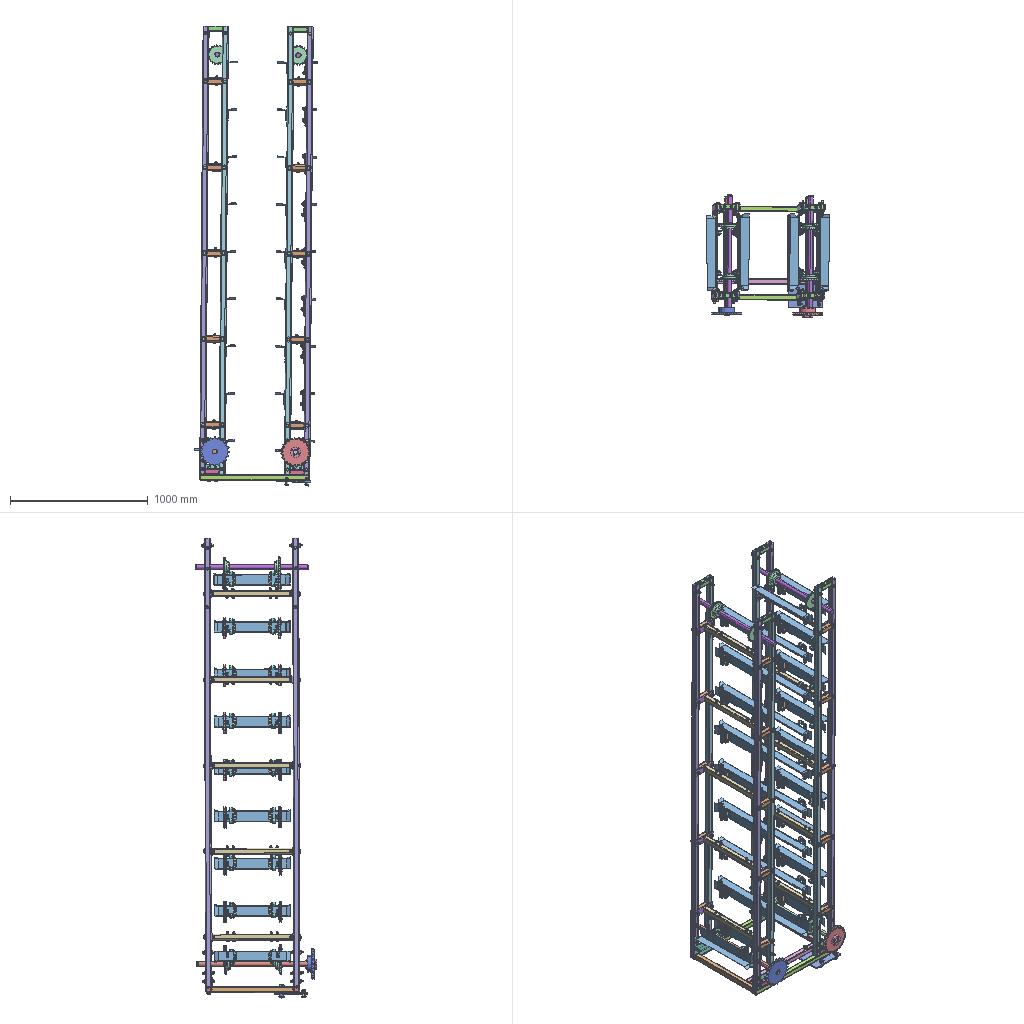Assembly | STEP file | 56 different items | 2795 placed | box 888 x 883 x 3334 mm
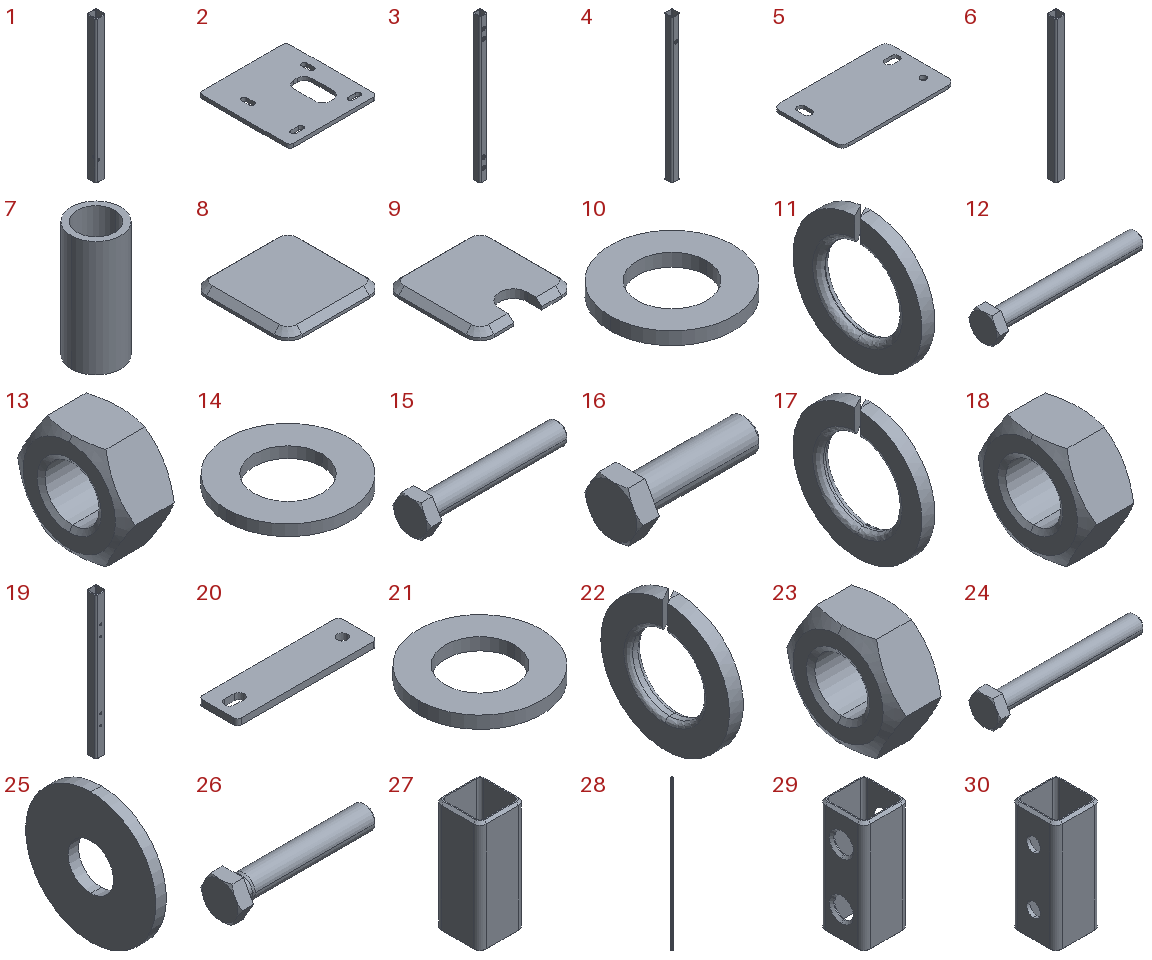Parts list (item | name | quantity | parent item | size | volume):
1 | IN-01-01-01-05 | x1 | in IN-01-01-01 | 40 x 40 x 590 mm | 239994 mm3
2 | IN-01-01-01-08 | x1 | in IN-01-01-01 | 240 x 250 x 10 mm | 535218 mm3
3 | IN-01-01-01-07 | x2 | in IN-01-01-01 | 40 x 40 x 795 mm | 317936 mm3
4 | IN-01-01-01-04 | x1 | in IN-01-01-01 | 40 x 40 x 715 mm | 290473 mm3
5 | IN-01-01-01-01 | x4 | in IN-01-01-01 | 180 x 110 x 5 mm | 95551 mm3
6 | IN-01-01-01-06 | x1 | in IN-01-01-01 | 40 x 40 x 590 mm | 240323 mm3
7 | IN-01-01-01-09 | x28 | in IN-01-01-01, IN-01-01-04 | 17.2 x 17.2 x 40 mm | 3820 mm3
8 | IN-01-01-01-03 | x10 | in IN-01-01-01, IN-01-01-04 | 34 x 34 x 3 mm | 3157 mm3
9 | IN-01-01-01-02 | x2 | in IN-01-01-01 | 34 x 34 x 3 mm | 2909 mm3
10 | DIN 126 - 13,5 | x120 | in IN-01-01-01, IN-01-01-03, IN-01-01-04 | 24 x 24 x 2.5 mm | 773.126 mm3
11 | DIN 128 - A12 | x80 | in IN-01-01-01, IN-01-01-03, IN-01-01-04 | 2.1 x 21.1 x 21.1 mm | 443.515 mm3
12 | DIN 931-1 - M12 x 100 | x8 | in IN-01-01-01 | 107.5 x 21.939 x 19 mm | 13582 mm3
13 | DIN 934 - M12 x 1,75 | x80 | in IN-01-01-01, IN-01-01-03, IN-01-01-04 | 10 x 21.939 x 19 mm | 2235 mm3
14 | DIN 126 - 15,5 | x8 | in IN-01-01-01 | 28 x 28 x 2.5 mm | 1068 mm3
15 | DIN 931-1 - M14 x 90 | x2 | in IN-01-01-01 | 98.8 x 25.403 x 22 mm | 17447 mm3
16 | DIN 931-1 - M14 x 50 | x2 | in IN-01-01-01 | 58.8 x 25.403 x 22 mm | 11289 mm3
17 | DIN 128 - A14 | x4 | in IN-01-01-01 | 2.4 x 24.1 x 24.1 mm | 656.657 mm3
18 | DIN 934 - M14 x 2 | x4 | in IN-01-01-01 | 11 x 25.403 x 22 mm | 3279 mm3
19 | IN-01-01-03-01 | x10 | in IN-01-01-03 | 40 x 40 x 584 mm | 236623 mm3
20 | IN-01-01-03-02 | x20 | in IN-01-01-03 | 180 x 50 x 8 mm | 68457 mm3
21 | DIN 126 - 9 | x80 | in IN-01-01-03 | 16 x 16 x 1.6 mm | 219.911 mm3
22 | DIN 128 - A8 | x40 | in IN-01-01-03 | 1.6 x 14.8 x 14.8 mm | 178.354 mm3
23 | DIN 934 - M8 x 1,25 | x40 | in IN-01-01-03 | 6.5 x 15.011 x 13 mm | 685.44 mm3
24 | DIN 931-1 - M8 x 65 | x40 | in IN-01-01-03 | 70.3 x 15.011 x 13 mm | 4009 mm3
25 | DIN 9021 - 13 | x40 | in IN-01-01-03 | 3 x 37 x 37 mm | 2827 mm3
26 | DIN 933 - M12  x 70 | x40 | in IN-01-01-03 | 77.5 x 21.939 x 19 mm | 10105 mm3
27 | IN-01-01-04-03 | x20 | in IN-01-01-04 | 40 x 40 x 100 mm | 40287 mm3
28 | IN-01-01-04-02 | x4 | in IN-01-01-04 | 40 x 40 x 3250 mm | 1317285 mm3
29 | IN-01-01-04-05 | x4 | in IN-01-01-04 | 40 x 40 x 100 mm | 37023 mm3
30 | IN-01-01-04-04 | x4 | in IN-01-01-04 | 40 x 40 x 100 mm | 38931 mm3
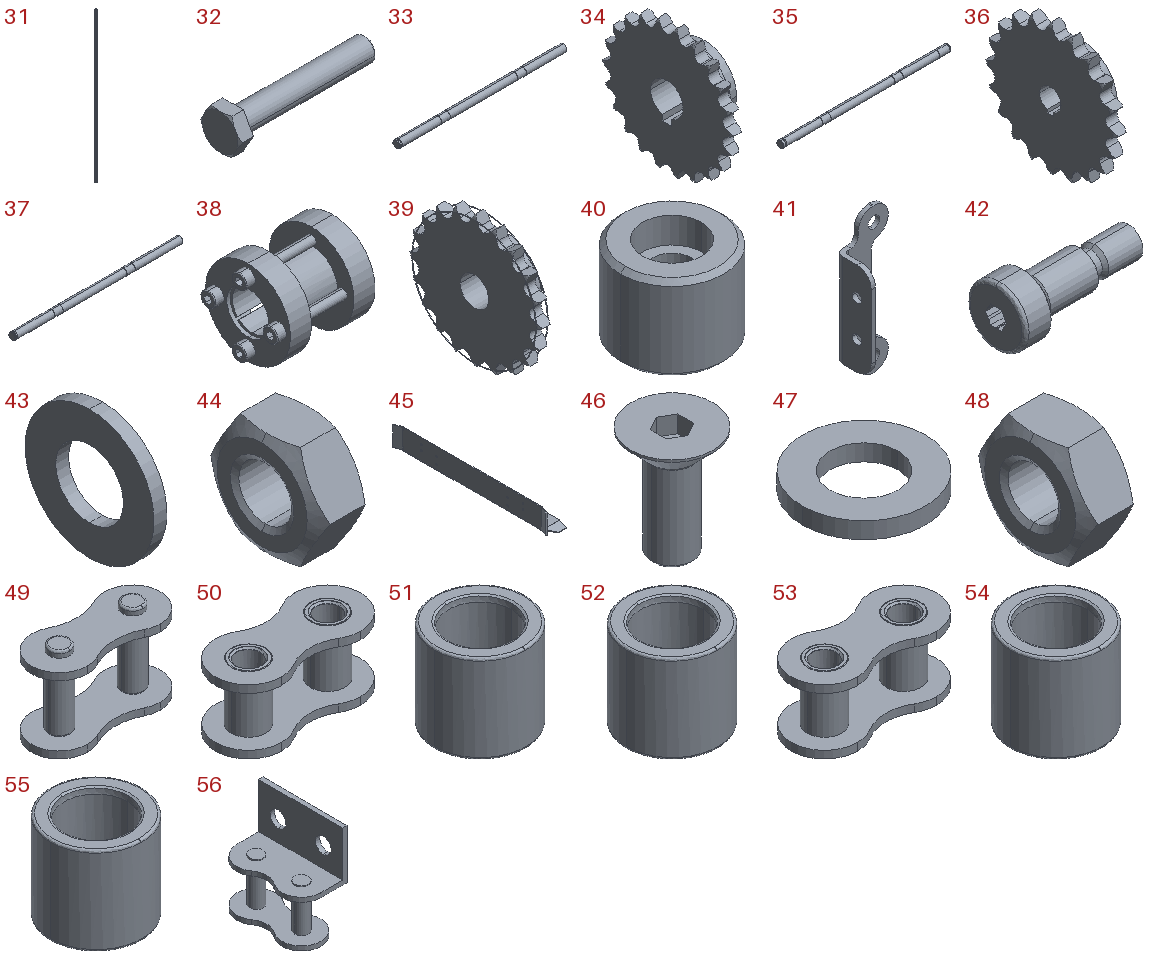31 | IN-01-01-04-01 | x4 | in IN-01-01-04 | 40 x 40 x 3250 mm | 1322181 mm3
32 | DIN 931-1 - M12 x 70 | x32 | in IN-01-01-04 | 77.5 x 21.939 x 19 mm | 10189 mm3
33 | IN-01-09-01 | x2 | in IN-01-09 | 816.1 x 35 x 35 mm | 780993 mm3
34 | IN-01-09-02 | x8 | in IN-01-09, IN-01-20, IN-01-21 | 40 x 141.8 x 140.357 mm | 249105 mm3
35 | IN-01-20-01_1 | x1 | in IN-01-20-01 | 865 x 35 x 35 mm | 826460 mm3
36 | IN-01-20-02 | x1 | in IN-01-20 | 50 x 218.1 x 218.1 mm | 860635 mm3
37 | IN-01-21-01 | x1 | in IN-01-21 | 865 x 35 x 35 mm | 828041 mm3
38 | IN-01-21-03 | x1 | in IN-01-21-02 | 83 x 75 x 75 mm | 165688 mm3
39 | IN-01-21-02_1 | x1 | in IN-01-21-02 | - | -
40 | IN-01-08-01-02-02 | x112 | in IN-01-08-01-02 | 28 x 28 x 23 mm | 11236 mm3
41 | IN-01-08-01-02-01 | x56 | in IN-01-08-01-02 | 34 x 25 x 101 mm | 9812 mm3
42 | ANSI B18.3.3M - M8x1,25 x 29,25 | x112 | in IN-01-08-01-02 | 36.25 x 16 x 16 mm | 3128 mm3
43 | DIN 125-2 - B 8,4 | x112 | in IN-01-08-01-02 | 1.6 x 16 x 16 mm | 233.031 mm3
44 | DIN 934 - M8 | x112 | in IN-01-08-01-02 | 6.5 x 15.011 x 13 mm | 685.44 mm3
45 | IN-01-08-01-01_1 | x28 | in IN-01-08-01-01 | 74.017 x 548.705 x 83.447 mm | 217025 mm3
46 | DIN 7991 - M6x16 | x224 | in IN-01-08-01-01, IN-01-08-01 | 12 x 12 x 16 mm | 554.104 mm3
47 | DIN 126 - 6,6 | x224 | in IN-01-08-01-01, IN-01-08-01 | 12 x 12 x 1.6 mm | 126.217 mm3
48 | DIN 934 - M6 x 1 | x224 | in IN-01-08-01-01, IN-01-08-01 | 5 x 11.547 x 10 mm | 321.226 mm3
49 | 12b-1_01 | x112 | in IN_01_01_07_01_02 | 33.5 x 14.5 x 22.6 mm | 2362 mm3
50 | 12b-1_02 | x112 | in IN_01_01_07_01_02 | 35 x 15.9 x 15.6 mm | 2056 mm3
51 | 12b-1_03 | x112 | in IN_01_01_07_01_02 | 12.07 x 12.07 x 11.6 mm | 689.728 mm3
52 | 12b-1_04 | x112 | in IN_01_01_07_01_02 | 12.07 x 12.07 x 11.6 mm | 689.728 mm3
53 | 12b-1_05 | x112 | in IN_01_01_07_01_02 | 35 x 15.9 x 15.6 mm | 2056 mm3
54 | 12b-1_06 | x112 | in IN_01_01_07_01_02 | 12.07 x 12.07 x 11.6 mm | 689.728 mm3
55 | 12b-1_07 | x112 | in IN_01_01_07_01_02 | 12.07 x 12.07 x 11.6 mm | 689.728 mm3
56 | IN_01_01_07_01_03 | x56 | in IN-01-08-01-02_1 | 19.15 x 35.35 x 39.1 mm | 3982 mm3
Placements (level | parent | child | x y z in mm | rotation matrix by rows), first 376 of 3099 lines:
1 | subassembly 2 | R1 | 7951.862 -633.159 955.539 | 1 0 0 0 1 0 0 0 1
2 | R1 | IN-01-01-01 | -8275.879 162.941 -2741.192 | -0.005068 -0.007537 1 -1 -0.002503 -0.005087 0.002541 -1 -0.007524
3 | IN-01-01-01 | IN-01-01-01-05 | -169.23 -114.088 623.28 | 0 0 -1 0 1 0 1 0 0
3 | IN-01-01-01 | IN-01-01-01-08 | -369.23 -94.088 343.28 | 1 0 0 0 0 1 0 -1 -0
3 | IN-01-01-01 | IN-01-01-01-07 | -784.23 -114.088 -111.72 | 1 0 0 0 1 0 0 0 1
3 | IN-01-01-01 | IN-01-01-01-07 | -144.23 -114.088 683.28 | -1 0 0 0 1 0 0 0 -1
3 | IN-01-01-01 | IN-01-01-01-04 | -259.23 -114.088 -71.72 | 1 0 0 0 1 0 0 0 1
3 | IN-01-01-01 | IN-01-01-01-01 | -164.23 -204.088 68.28 | 0 0 -1 0 -1 0 -1 0 0
3 | IN-01-01-01 | IN-01-01-01-01 | -169.23 -204.088 503.28 | 0 0 1 0 -1 0 1 0 -0
3 | IN-01-01-01 | IN-01-01-01-01 | -764.23 -204.088 503.28 | 0 0 1 0 -1 0 1 0 -0
3 | IN-01-01-01 | IN-01-01-01-01 | -759.23 -204.088 68.28 | 0 0 -1 0 -1 0 -1 0 0
3 | IN-01-01-01 | IN-01-01-01-06 | -169.23 -114.088 -91.72 | 0 0 -1 0 1 0 1 0 0
3 | IN-01-01-01 | IN-01-01-01-09 | -784.23 -134.088 -46.72 | 1 0 0 0 0 1 0 -1 0
3 | IN-01-01-01 | IN-01-01-01-09 | -784.23 -134.088 3.28 | 1 0 0 0 0 1 0 -1 0
3 | IN-01-01-01 | IN-01-01-01-09 | -784.23 -134.088 618.28 | 1 0 0 0 0 1 0 -1 0
3 | IN-01-01-01 | IN-01-01-01-09 | -144.23 -134.088 3.28 | 1 0 0 0 0 1 0 -1 0
3 | IN-01-01-01 | IN-01-01-01-09 | -144.23 -134.088 618.28 | 1 0 0 0 0 1 0 -1 0
3 | IN-01-01-01 | IN-01-01-01-09 | -144.23 -134.088 568.28 | 1 0 0 0 0 1 0 -1 0
3 | IN-01-01-01 | IN-01-01-01-09 | -144.23 -134.088 -46.72 | 1 0 0 0 0 1 0 -1 0
3 | IN-01-01-01 | IN-01-01-01-09 | -784.23 -134.088 568.28 | 1 0 0 0 0 1 0 -1 0
3 | IN-01-01-01 | IN-01-01-01-03 | -161.33 -131.188 680.28 | 0 -1 0 1 0 0 0 0 1
3 | IN-01-01-01 | IN-01-01-01-02 | -127.13 -97.188 -108.72 | -1 0 0 0 1 0 0 0 -1
3 | IN-01-01-01 | IN-01-01-01-03 | -801.33 -131.188 680.28 | 0 -1 0 1 0 0 0 0 1
3 | IN-01-01-01 | IN-01-01-01-02 | -767.33 -97.188 -108.72 | -1 0 0 0 1 0 0 0 -1
3 | IN-01-01-01 | DIN 126 - 13,5 | -784.23 -91.588 568.28 | -1 0 0 0 0 1 0 1 0
3 | IN-01-01-01 | DIN 126 - 13,5 | -784.23 -91.588 -46.72 | -1 0 0 0 0 1 0 1 0
3 | IN-01-01-01 | DIN 126 - 13,5 | -784.23 -91.588 3.28 | -1 0 0 0 0 1 0 1 0
3 | IN-01-01-01 | DIN 126 - 13,5 | -784.23 -91.588 618.28 | -1 0 0 0 0 1 0 1 0
3 | IN-01-01-01 | DIN 126 - 13,5 | -144.23 -91.588 3.28 | -1 0 0 0 0 1 0 1 0
3 | IN-01-01-01 | DIN 126 - 13,5 | -144.23 -91.588 618.28 | -1 0 0 0 0 1 0 1 0
3 | IN-01-01-01 | DIN 126 - 13,5 | -144.23 -91.588 568.28 | -1 0 0 0 0 1 0 1 0
3 | IN-01-01-01 | DIN 126 - 13,5 | -144.23 -91.588 -46.72 | -1 0 0 0 0 1 0 1 0
3 | IN-01-01-01 | DIN 126 - 13,5 | -144.23 -176.588 618.28 | 1 0 0 0 0 -1 0 1 -0
3 | IN-01-01-01 | DIN 126 - 13,5 | -144.23 -176.588 -46.72 | 1 0 0 0 0 -1 0 1 -0
3 | IN-01-01-01 | DIN 126 - 13,5 | -144.23 -176.588 3.28 | 1 0 0 0 0 -1 0 1 -0
3 | IN-01-01-01 | DIN 126 - 13,5 | -144.23 -176.588 568.28 | 1 0 0 0 0 -1 0 1 -0
3 | IN-01-01-01 | DIN 126 - 13,5 | -784.23 -176.588 618.28 | 1 0 0 0 0 -1 0 1 -0
3 | IN-01-01-01 | DIN 126 - 13,5 | -784.23 -176.588 568.28 | 1 0 0 0 0 -1 0 1 -0
3 | IN-01-01-01 | DIN 126 - 13,5 | -784.23 -176.588 3.28 | 1 0 0 0 0 -1 0 1 -0
3 | IN-01-01-01 | DIN 126 - 13,5 | -784.23 -176.588 -46.72 | 1 0 0 0 0 -1 0 1 -0
3 | IN-01-01-01 | DIN 128 - A12 | -144.23 -176.588 618.28 | 0 1 0 -1 0 0 0 0 1
3 | IN-01-01-01 | DIN 128 - A12 | -144.23 -176.588 568.28 | 0 1 0 -1 0 0 0 0 1
3 | IN-01-01-01 | DIN 128 - A12 | -144.23 -176.588 3.28 | 0 1 0 -1 0 0 0 0 1
3 | IN-01-01-01 | DIN 128 - A12 | -144.23 -176.588 -46.72 | 0 1 0 -1 0 0 0 0 1
3 | IN-01-01-01 | DIN 128 - A12 | -784.23 -176.588 -46.72 | 0 1 0 -1 0 0 0 0 1
3 | IN-01-01-01 | DIN 128 - A12 | -784.23 -176.588 3.28 | 0 1 0 -1 0 0 0 0 1
3 | IN-01-01-01 | DIN 128 - A12 | -784.23 -176.588 568.28 | 0 1 0 -1 0 0 0 0 1
3 | IN-01-01-01 | DIN 128 - A12 | -784.23 -176.588 618.28 | 0 1 0 -1 0 0 0 0 1
3 | IN-01-01-01 | DIN 931-1 - M12 x 100 | -784.23 -91.588 -46.72 | 0 1 0 -1 0 0 0 0 1
3 | IN-01-01-01 | DIN 931-1 - M12 x 100 | -784.23 -91.588 3.28 | 0 1 0 -1 0 0 0 0 1
3 | IN-01-01-01 | DIN 931-1 - M12 x 100 | -784.23 -91.588 568.28 | 0 1 0 -1 0 0 0 0 1
3 | IN-01-01-01 | DIN 931-1 - M12 x 100 | -784.23 -91.588 618.28 | 0 1 0 -1 0 0 0 0 1
3 | IN-01-01-01 | DIN 931-1 - M12 x 100 | -144.23 -91.588 618.28 | 0 1 0 -1 0 0 0 0 1
3 | IN-01-01-01 | DIN 931-1 - M12 x 100 | -144.23 -91.588 568.28 | 0 1 0 -1 0 0 0 0 1
3 | IN-01-01-01 | DIN 931-1 - M12 x 100 | -144.23 -91.588 3.28 | 0 1 0 -1 0 0 0 0 1
3 | IN-01-01-01 | DIN 931-1 - M12 x 100 | -144.23 -91.588 -46.72 | 0 1 0 -1 0 0 0 0 1
3 | IN-01-01-01 | DIN 934 - M12 x 1,75 | -144.23 -188.688 618.28 | 0 -1 0 1 0 0 0 0 1
3 | IN-01-01-01 | DIN 934 - M12 x 1,75 | -144.23 -188.688 568.28 | 0 -1 0 1 0 0 0 0 1
3 | IN-01-01-01 | DIN 934 - M12 x 1,75 | -144.23 -188.688 3.28 | 0 -1 0 1 0 0 0 0 1
3 | IN-01-01-01 | DIN 934 - M12 x 1,75 | -144.23 -188.688 -46.72 | 0 -1 0 1 0 0 0 0 1
3 | IN-01-01-01 | DIN 934 - M12 x 1,75 | -784.23 -188.688 -46.72 | 0 -1 0 1 0 0 0 0 1
3 | IN-01-01-01 | DIN 934 - M12 x 1,75 | -784.23 -188.688 3.28 | 0 -1 0 1 0 0 0 0 1
3 | IN-01-01-01 | DIN 934 - M12 x 1,75 | -784.23 -188.688 568.28 | 0 -1 0 1 0 0 0 0 1
3 | IN-01-01-01 | DIN 934 - M12 x 1,75 | -784.23 -188.688 618.28 | 0 -1 0 1 0 0 0 0 1
3 | IN-01-01-01 | DIN 126 - 15,5 | -261.73 -64.588 520.78 | -1 0 0 0 0 1 0 1 -0
3 | IN-01-01-01 | DIN 126 - 15,5 | -251.73 -64.588 665.78 | -1 0 0 0 0 1 0 1 -0
3 | IN-01-01-01 | DIN 126 - 15,5 | -93.73 -64.588 665.78 | -1 0 0 0 0 1 0 1 -0
3 | IN-01-01-01 | DIN 126 - 15,5 | -96.73 -64.588 520.78 | -1 0 0 0 0 1 0 1 -0
3 | IN-01-01-01 | DIN 931-1 - M14 x 90 | -261.73 -64.588 520.78 | 0 1 0 -1 0 0 0 0 1
3 | IN-01-01-01 | DIN 931-1 - M14 x 90 | -251.73 -64.588 665.78 | 0 1 0 -1 0 0 0 0 1
3 | IN-01-01-01 | DIN 931-1 - M14 x 50 | -93.73 -64.588 665.78 | 0 1 0 -1 0 0 0 0 1
3 | IN-01-01-01 | DIN 931-1 - M14 x 50 | -96.73 -64.588 520.78 | 0 1 0 -1 0 0 0 0 1
3 | IN-01-01-01 | DIN 126 - 15,5 | -93.73 -96.588 665.78 | 1 0 0 0 0 -1 0 1 -0
3 | IN-01-01-01 | DIN 126 - 15,5 | -251.73 -136.588 665.78 | 1 0 0 0 0 -1 0 1 -0
3 | IN-01-01-01 | DIN 126 - 15,5 | -261.73 -136.588 520.78 | 1 0 0 0 0 -1 0 1 -0
3 | IN-01-01-01 | DIN 126 - 15,5 | -96.73 -96.588 520.78 | 1 0 0 0 0 -1 0 1 -0
3 | IN-01-01-01 | DIN 128 - A14 | -93.73 -96.588 665.78 | 0 1 0 -1 0 0 0 0 1
3 | IN-01-01-01 | DIN 128 - A14 | -251.73 -136.588 665.78 | 0 1 0 -1 0 0 0 0 1
3 | IN-01-01-01 | DIN 128 - A14 | -261.73 -136.588 520.78 | 0 1 0 -1 0 0 0 0 1
3 | IN-01-01-01 | DIN 128 - A14 | -96.73 -96.588 520.78 | 0 1 0 -1 0 0 0 0 1
3 | IN-01-01-01 | DIN 934 - M14 x 2 | -96.73 -109.988 520.78 | 0 -1 0 1 0 0 0 0 1
3 | IN-01-01-01 | DIN 934 - M14 x 2 | -93.73 -109.988 665.78 | 0 -1 0 1 0 0 0 0 1
3 | IN-01-01-01 | DIN 934 - M14 x 2 | -251.73 -149.988 665.78 | 0 -1 0 1 0 0 0 0 1
3 | IN-01-01-01 | DIN 934 - M14 x 2 | -261.73 -149.988 520.78 | 0 -1 0 1 0 0 0 0 1
2 | R1 | IN-01-01-03 | -8254.616 637.893 -1630.668 | 1 -0.007537 0.005068 -0.005087 -0.002503 1 -0.007524 -1 -0.002541
3 | IN-01-01-03 | IN-01-01-03-01 | -22.21 -4.25 -300.0 | 1 0 0 0 1 0 0 0 1
3 | IN-01-01-03 | IN-01-01-03-02 | -122.21 20.75 284.0 | 1 0 0 0 1 0 0 0 1
3 | IN-01-01-03 | IN-01-01-03-02 | -122.21 -29.25 -300.0 | 1 0 0 0 -1 0 0 0 -1
3 | IN-01-01-03 | DIN 126 - 9 | -22.21 21.35 172.0 | -1 0 0 0 0 1 0 1 0
3 | IN-01-01-03 | DIN 126 - 9 | -22.21 21.35 -144.0 | -1 0 0 0 0 1 0 1 0
3 | IN-01-01-03 | DIN 126 - 9 | -22.21 21.35 128.0 | -1 0 0 0 0 1 0 1 0
3 | IN-01-01-03 | DIN 126 - 9 | -22.21 21.35 -188.0 | -1 0 0 0 0 1 0 1 0
3 | IN-01-01-03 | DIN 126 - 9 | -22.21 -29.85 172.0 | 1 0 0 0 0 -1 0 1 0
3 | IN-01-01-03 | DIN 126 - 9 | -22.21 -29.85 -144.0 | 1 0 0 0 0 -1 0 1 0
3 | IN-01-01-03 | DIN 126 - 9 | -22.21 -29.85 128.0 | 1 0 0 0 0 -1 0 1 0
3 | IN-01-01-03 | DIN 126 - 9 | -22.21 -29.85 -188.0 | 1 0 0 0 0 -1 0 1 0
3 | IN-01-01-03 | DIN 128 - A8 | -22.21 -29.85 172.0 | 0 1 0 -1 0 0 0 0 1
3 | IN-01-01-03 | DIN 128 - A8 | -22.21 -29.85 -144.0 | 0 1 0 -1 0 0 0 0 1
3 | IN-01-01-03 | DIN 128 - A8 | -22.21 -29.85 128.0 | 0 1 0 -1 0 0 0 0 1
3 | IN-01-01-03 | DIN 128 - A8 | -22.21 -29.85 -188.0 | 0 1 0 -1 0 0 0 0 1
3 | IN-01-01-03 | DIN 934 - M8 x 1,25 | -22.21 -37.95 172.0 | 0 -1 0 1 0 0 0 0 1
3 | IN-01-01-03 | DIN 934 - M8 x 1,25 | -22.21 -37.95 128.0 | 0 -1 0 1 0 0 0 0 1
3 | IN-01-01-03 | DIN 934 - M8 x 1,25 | -22.21 -37.95 -144.0 | 0 -1 0 1 0 0 0 0 1
3 | IN-01-01-03 | DIN 934 - M8 x 1,25 | -22.21 -37.95 -188.0 | 0 -1 0 1 0 0 0 0 1
3 | IN-01-01-03 | DIN 931-1 - M8 x 65 | -22.21 21.35 172.0 | 0 1 0 -1 0 0 0 0 1
3 | IN-01-01-03 | DIN 931-1 - M8 x 65 | -22.21 21.35 -144.0 | 0 1 0 -1 0 0 0 0 1
3 | IN-01-01-03 | DIN 931-1 - M8 x 65 | -22.21 21.35 128.0 | 0 1 0 -1 0 0 0 0 1
3 | IN-01-01-03 | DIN 931-1 - M8 x 65 | -22.21 21.35 -188.0 | 0 1 0 -1 0 0 0 0 1
3 | IN-01-01-03 | DIN 126 - 13,5 | 37.79 -4.25 -297.5 | 1 0 0 0 1 0 0 0 1
3 | IN-01-01-03 | DIN 126 - 13,5 | -101.163 -3.5 -297.5 | 0.9495 -0.3138 0 0.3138 0.9495 0 0 0 1
3 | IN-01-01-03 | DIN 126 - 13,5 | 37.79 -4.25 281.5 | -1 0 0 0 1 0 0 0 -1
3 | IN-01-01-03 | DIN 126 - 13,5 | -101.163 -3.5 281.5 | -0.9998 0.01923 0 0.01923 0.9998 0 0 0 -1
3 | IN-01-01-03 | DIN 9021 - 13 | 37.79 -4.25 332.0 | 0 1 0 0 0 1 1 0 0
3 | IN-01-01-03 | DIN 9021 - 13 | -101.163 -3.5 332.0 | 0 1 0 0 0 1 1 0 -0
3 | IN-01-01-03 | DIN 9021 - 13 | 37.79 -4.25 -348.0 | 0 -1 0 0 0 1 -1 0 0
3 | IN-01-01-03 | DIN 9021 - 13 | -101.163 -3.5 -348.0 | 0 -0.9113 -0.4118 0 -0.4118 0.9113 -1 0 0
3 | IN-01-01-03 | DIN 128 - A12 | 37.79 -4.25 281.5 | 0 1 0 0 0 -1 -1 0 0
3 | IN-01-01-03 | DIN 128 - A12 | -101.163 -3.5 281.5 | 0 -0.9778 -0.2094 0 -0.2094 0.9778 -1 0 0
3 | IN-01-01-03 | DIN 128 - A12 | -101.163 -3.5 -297.5 | 0 0.9553 -0.2958 0 0.2958 0.9553 1 0 0
3 | IN-01-01-03 | DIN 128 - A12 | 37.79 -4.25 -297.5 | 0 1 0 0 0 1 1 0 0
3 | IN-01-01-03 | DIN 933 - M12  x 70 | 37.79 -4.25 -351.0 | 0 1 0 0 0 1 1 0 0
3 | IN-01-01-03 | DIN 933 - M12  x 70 | -101.163 -3.5 -351.0 | 0 1 0 0 0 1 1 0 0
3 | IN-01-01-03 | DIN 933 - M12  x 70 | 37.79 -4.25 335.0 | 0 -1 0 0 0 1 -1 0 0
3 | IN-01-01-03 | DIN 933 - M12  x 70 | -101.163 -3.5 335.0 | 0 -1 0 0 0 1 -1 0 -0
3 | IN-01-01-03 | DIN 934 - M12 x 1,75 | -101.163 -3.5 -285.4 | 0 -1 0 0 0 1 -1 0 0
3 | IN-01-01-03 | DIN 934 - M12 x 1,75 | 37.79 -4.25 -285.4 | 0 -1 0 0 0 1 -1 0 0
3 | IN-01-01-03 | DIN 934 - M12 x 1,75 | -101.163 -3.5 269.4 | 0 1 0 0 0 1 1 0 0
3 | IN-01-01-03 | DIN 934 - M12 x 1,75 | 37.79 -4.25 269.4 | 0 1 0 0 0 1 1 0 0
2 | R1 | IN-01-01-03 | -8259.304 636.336 -2252.648 | 1 -0.007537 0.005068 -0.005087 -0.002503 1 -0.007524 -1 -0.002541
3 | IN-01-01-03 | IN-01-01-03-01 | -22.21 -4.25 -300.0 | 1 0 0 0 1 0 0 0 1
3 | IN-01-01-03 | IN-01-01-03-02 | -122.21 20.75 284.0 | 1 0 0 0 1 0 0 0 1
3 | IN-01-01-03 | IN-01-01-03-02 | -122.21 -29.25 -300.0 | 1 0 0 0 -1 0 0 0 -1
3 | IN-01-01-03 | DIN 126 - 9 | -22.21 21.35 172.0 | -1 0 0 0 0 1 0 1 0
3 | IN-01-01-03 | DIN 126 - 9 | -22.21 21.35 -144.0 | -1 0 0 0 0 1 0 1 0
3 | IN-01-01-03 | DIN 126 - 9 | -22.21 21.35 128.0 | -1 0 0 0 0 1 0 1 0
3 | IN-01-01-03 | DIN 126 - 9 | -22.21 21.35 -188.0 | -1 0 0 0 0 1 0 1 0
3 | IN-01-01-03 | DIN 126 - 9 | -22.21 -29.85 172.0 | 1 0 0 0 0 -1 0 1 0
3 | IN-01-01-03 | DIN 126 - 9 | -22.21 -29.85 -144.0 | 1 0 0 0 0 -1 0 1 0
3 | IN-01-01-03 | DIN 126 - 9 | -22.21 -29.85 128.0 | 1 0 0 0 0 -1 0 1 0
3 | IN-01-01-03 | DIN 126 - 9 | -22.21 -29.85 -188.0 | 1 0 0 0 0 -1 0 1 0
3 | IN-01-01-03 | DIN 128 - A8 | -22.21 -29.85 172.0 | 0 1 0 -1 0 0 0 0 1
3 | IN-01-01-03 | DIN 128 - A8 | -22.21 -29.85 -144.0 | 0 1 0 -1 0 0 0 0 1
3 | IN-01-01-03 | DIN 128 - A8 | -22.21 -29.85 128.0 | 0 1 0 -1 0 0 0 0 1
3 | IN-01-01-03 | DIN 128 - A8 | -22.21 -29.85 -188.0 | 0 1 0 -1 0 0 0 0 1
3 | IN-01-01-03 | DIN 934 - M8 x 1,25 | -22.21 -37.95 172.0 | 0 -1 0 1 0 0 0 0 1
3 | IN-01-01-03 | DIN 934 - M8 x 1,25 | -22.21 -37.95 128.0 | 0 -1 0 1 0 0 0 0 1
3 | IN-01-01-03 | DIN 934 - M8 x 1,25 | -22.21 -37.95 -144.0 | 0 -1 0 1 0 0 0 0 1
3 | IN-01-01-03 | DIN 934 - M8 x 1,25 | -22.21 -37.95 -188.0 | 0 -1 0 1 0 0 0 0 1
3 | IN-01-01-03 | DIN 931-1 - M8 x 65 | -22.21 21.35 172.0 | 0 1 0 -1 0 0 0 0 1
3 | IN-01-01-03 | DIN 931-1 - M8 x 65 | -22.21 21.35 -144.0 | 0 1 0 -1 0 0 0 0 1
3 | IN-01-01-03 | DIN 931-1 - M8 x 65 | -22.21 21.35 128.0 | 0 1 0 -1 0 0 0 0 1
3 | IN-01-01-03 | DIN 931-1 - M8 x 65 | -22.21 21.35 -188.0 | 0 1 0 -1 0 0 0 0 1
3 | IN-01-01-03 | DIN 126 - 13,5 | 37.79 -4.25 -297.5 | 1 0 0 0 1 0 0 0 1
3 | IN-01-01-03 | DIN 126 - 13,5 | -101.163 -3.5 -297.5 | 0.9495 -0.3138 0 0.3138 0.9495 0 0 0 1
3 | IN-01-01-03 | DIN 126 - 13,5 | 37.79 -4.25 281.5 | -1 0 0 0 1 0 0 0 -1
3 | IN-01-01-03 | DIN 126 - 13,5 | -101.163 -3.5 281.5 | -0.9998 0.01923 0 0.01923 0.9998 0 0 0 -1
3 | IN-01-01-03 | DIN 9021 - 13 | 37.79 -4.25 332.0 | 0 1 0 0 0 1 1 0 0
3 | IN-01-01-03 | DIN 9021 - 13 | -101.163 -3.5 332.0 | 0 1 0 0 0 1 1 0 -0
3 | IN-01-01-03 | DIN 9021 - 13 | 37.79 -4.25 -348.0 | 0 -1 0 0 0 1 -1 0 0
3 | IN-01-01-03 | DIN 9021 - 13 | -101.163 -3.5 -348.0 | 0 -0.9113 -0.4118 0 -0.4118 0.9113 -1 0 0
3 | IN-01-01-03 | DIN 128 - A12 | 37.79 -4.25 281.5 | 0 1 0 0 0 -1 -1 0 0
3 | IN-01-01-03 | DIN 128 - A12 | -101.163 -3.5 281.5 | 0 -0.9778 -0.2094 0 -0.2094 0.9778 -1 0 0
3 | IN-01-01-03 | DIN 128 - A12 | -101.163 -3.5 -297.5 | 0 0.9553 -0.2958 0 0.2958 0.9553 1 0 0
3 | IN-01-01-03 | DIN 128 - A12 | 37.79 -4.25 -297.5 | 0 1 0 0 0 1 1 0 0
3 | IN-01-01-03 | DIN 933 - M12  x 70 | 37.79 -4.25 -351.0 | 0 1 0 0 0 1 1 0 0
3 | IN-01-01-03 | DIN 933 - M12  x 70 | -101.163 -3.5 -351.0 | 0 1 0 0 0 1 1 0 0
3 | IN-01-01-03 | DIN 933 - M12  x 70 | 37.79 -4.25 335.0 | 0 -1 0 0 0 1 -1 0 0
3 | IN-01-01-03 | DIN 933 - M12  x 70 | -101.163 -3.5 335.0 | 0 -1 0 0 0 1 -1 0 -0
3 | IN-01-01-03 | DIN 934 - M12 x 1,75 | -101.163 -3.5 -285.4 | 0 -1 0 0 0 1 -1 0 0
3 | IN-01-01-03 | DIN 934 - M12 x 1,75 | 37.79 -4.25 -285.4 | 0 -1 0 0 0 1 -1 0 0
3 | IN-01-01-03 | DIN 934 - M12 x 1,75 | -101.163 -3.5 269.4 | 0 1 0 0 0 1 1 0 0
3 | IN-01-01-03 | DIN 934 - M12 x 1,75 | 37.79 -4.25 269.4 | 0 1 0 0 0 1 1 0 0
2 | R1 | IN-01-01-03 | -8249.928 639.45 -1008.688 | 1 -0.007537 0.005068 -0.005087 -0.002503 1 -0.007524 -1 -0.002541
3 | IN-01-01-03 | IN-01-01-03-01 | -22.21 -4.25 -300.0 | 1 0 0 0 1 0 0 0 1
3 | IN-01-01-03 | IN-01-01-03-02 | -122.21 20.75 284.0 | 1 0 0 0 1 0 0 0 1
3 | IN-01-01-03 | IN-01-01-03-02 | -122.21 -29.25 -300.0 | 1 0 0 0 -1 0 0 0 -1
3 | IN-01-01-03 | DIN 126 - 9 | -22.21 21.35 172.0 | -1 0 0 0 0 1 0 1 0
3 | IN-01-01-03 | DIN 126 - 9 | -22.21 21.35 -144.0 | -1 0 0 0 0 1 0 1 0
3 | IN-01-01-03 | DIN 126 - 9 | -22.21 21.35 128.0 | -1 0 0 0 0 1 0 1 0
3 | IN-01-01-03 | DIN 126 - 9 | -22.21 21.35 -188.0 | -1 0 0 0 0 1 0 1 0
3 | IN-01-01-03 | DIN 126 - 9 | -22.21 -29.85 172.0 | 1 0 0 0 0 -1 0 1 0
3 | IN-01-01-03 | DIN 126 - 9 | -22.21 -29.85 -144.0 | 1 0 0 0 0 -1 0 1 0
3 | IN-01-01-03 | DIN 126 - 9 | -22.21 -29.85 128.0 | 1 0 0 0 0 -1 0 1 0
3 | IN-01-01-03 | DIN 126 - 9 | -22.21 -29.85 -188.0 | 1 0 0 0 0 -1 0 1 0
3 | IN-01-01-03 | DIN 128 - A8 | -22.21 -29.85 172.0 | 0 1 0 -1 0 0 0 0 1
3 | IN-01-01-03 | DIN 128 - A8 | -22.21 -29.85 -144.0 | 0 1 0 -1 0 0 0 0 1
3 | IN-01-01-03 | DIN 128 - A8 | -22.21 -29.85 128.0 | 0 1 0 -1 0 0 0 0 1
3 | IN-01-01-03 | DIN 128 - A8 | -22.21 -29.85 -188.0 | 0 1 0 -1 0 0 0 0 1
3 | IN-01-01-03 | DIN 934 - M8 x 1,25 | -22.21 -37.95 172.0 | 0 -1 0 1 0 0 0 0 1
3 | IN-01-01-03 | DIN 934 - M8 x 1,25 | -22.21 -37.95 128.0 | 0 -1 0 1 0 0 0 0 1
3 | IN-01-01-03 | DIN 934 - M8 x 1,25 | -22.21 -37.95 -144.0 | 0 -1 0 1 0 0 0 0 1
3 | IN-01-01-03 | DIN 934 - M8 x 1,25 | -22.21 -37.95 -188.0 | 0 -1 0 1 0 0 0 0 1
3 | IN-01-01-03 | DIN 931-1 - M8 x 65 | -22.21 21.35 172.0 | 0 1 0 -1 0 0 0 0 1
3 | IN-01-01-03 | DIN 931-1 - M8 x 65 | -22.21 21.35 -144.0 | 0 1 0 -1 0 0 0 0 1
3 | IN-01-01-03 | DIN 931-1 - M8 x 65 | -22.21 21.35 128.0 | 0 1 0 -1 0 0 0 0 1
3 | IN-01-01-03 | DIN 931-1 - M8 x 65 | -22.21 21.35 -188.0 | 0 1 0 -1 0 0 0 0 1
3 | IN-01-01-03 | DIN 126 - 13,5 | 37.79 -4.25 -297.5 | 1 0 0 0 1 0 0 0 1
3 | IN-01-01-03 | DIN 126 - 13,5 | -101.163 -3.5 -297.5 | 0.9495 -0.3138 0 0.3138 0.9495 0 0 0 1
3 | IN-01-01-03 | DIN 126 - 13,5 | 37.79 -4.25 281.5 | -1 0 0 0 1 0 0 0 -1
3 | IN-01-01-03 | DIN 126 - 13,5 | -101.163 -3.5 281.5 | -0.9998 0.01923 0 0.01923 0.9998 0 0 0 -1
3 | IN-01-01-03 | DIN 9021 - 13 | 37.79 -4.25 332.0 | 0 1 0 0 0 1 1 0 0
3 | IN-01-01-03 | DIN 9021 - 13 | -101.163 -3.5 332.0 | 0 1 0 0 0 1 1 0 -0
3 | IN-01-01-03 | DIN 9021 - 13 | 37.79 -4.25 -348.0 | 0 -1 0 0 0 1 -1 0 0
3 | IN-01-01-03 | DIN 9021 - 13 | -101.163 -3.5 -348.0 | 0 -0.9113 -0.4118 0 -0.4118 0.9113 -1 0 0
3 | IN-01-01-03 | DIN 128 - A12 | 37.79 -4.25 281.5 | 0 1 0 0 0 -1 -1 0 0
3 | IN-01-01-03 | DIN 128 - A12 | -101.163 -3.5 281.5 | 0 -0.9778 -0.2094 0 -0.2094 0.9778 -1 0 0
3 | IN-01-01-03 | DIN 128 - A12 | -101.163 -3.5 -297.5 | 0 0.9553 -0.2958 0 0.2958 0.9553 1 0 0
3 | IN-01-01-03 | DIN 128 - A12 | 37.79 -4.25 -297.5 | 0 1 0 0 0 1 1 0 0
3 | IN-01-01-03 | DIN 933 - M12  x 70 | 37.79 -4.25 -351.0 | 0 1 0 0 0 1 1 0 0
3 | IN-01-01-03 | DIN 933 - M12  x 70 | -101.163 -3.5 -351.0 | 0 1 0 0 0 1 1 0 0
3 | IN-01-01-03 | DIN 933 - M12  x 70 | 37.79 -4.25 335.0 | 0 -1 0 0 0 1 -1 0 0
3 | IN-01-01-03 | DIN 933 - M12  x 70 | -101.163 -3.5 335.0 | 0 -1 0 0 0 1 -1 0 -0
3 | IN-01-01-03 | DIN 934 - M12 x 1,75 | -101.163 -3.5 -285.4 | 0 -1 0 0 0 1 -1 0 0
3 | IN-01-01-03 | DIN 934 - M12 x 1,75 | 37.79 -4.25 -285.4 | 0 -1 0 0 0 1 -1 0 0
3 | IN-01-01-03 | DIN 934 - M12 x 1,75 | -101.163 -3.5 269.4 | 0 1 0 0 0 1 1 0 0
3 | IN-01-01-03 | DIN 934 - M12 x 1,75 | 37.79 -4.25 269.4 | 0 1 0 0 0 1 1 0 0
2 | R1 | IN-01-01-03 | -7704.14 619.092 -1634.77 | -1 -0.007537 -0.005068 0.005087 -0.002503 -1 0.007524 -1 0.002541
3 | IN-01-01-03 | IN-01-01-03-01 | -22.21 -4.25 -300.0 | 1 0 0 0 1 0 0 0 1
3 | IN-01-01-03 | IN-01-01-03-02 | -122.21 20.75 284.0 | 1 0 0 0 1 0 0 0 1
3 | IN-01-01-03 | IN-01-01-03-02 | -122.21 -29.25 -300.0 | 1 0 0 0 -1 0 0 0 -1
3 | IN-01-01-03 | DIN 126 - 9 | -22.21 21.35 172.0 | -1 0 0 0 0 1 0 1 0
3 | IN-01-01-03 | DIN 126 - 9 | -22.21 21.35 -144.0 | -1 0 0 0 0 1 0 1 0
3 | IN-01-01-03 | DIN 126 - 9 | -22.21 21.35 128.0 | -1 0 0 0 0 1 0 1 0
3 | IN-01-01-03 | DIN 126 - 9 | -22.21 21.35 -188.0 | -1 0 0 0 0 1 0 1 0
3 | IN-01-01-03 | DIN 126 - 9 | -22.21 -29.85 172.0 | 1 0 0 0 0 -1 0 1 0
3 | IN-01-01-03 | DIN 126 - 9 | -22.21 -29.85 -144.0 | 1 0 0 0 0 -1 0 1 0
3 | IN-01-01-03 | DIN 126 - 9 | -22.21 -29.85 128.0 | 1 0 0 0 0 -1 0 1 0
3 | IN-01-01-03 | DIN 126 - 9 | -22.21 -29.85 -188.0 | 1 0 0 0 0 -1 0 1 0
3 | IN-01-01-03 | DIN 128 - A8 | -22.21 -29.85 172.0 | 0 1 0 -1 0 0 0 0 1
3 | IN-01-01-03 | DIN 128 - A8 | -22.21 -29.85 -144.0 | 0 1 0 -1 0 0 0 0 1
3 | IN-01-01-03 | DIN 128 - A8 | -22.21 -29.85 128.0 | 0 1 0 -1 0 0 0 0 1
3 | IN-01-01-03 | DIN 128 - A8 | -22.21 -29.85 -188.0 | 0 1 0 -1 0 0 0 0 1
3 | IN-01-01-03 | DIN 934 - M8 x 1,25 | -22.21 -37.95 172.0 | 0 -1 0 1 0 0 0 0 1
3 | IN-01-01-03 | DIN 934 - M8 x 1,25 | -22.21 -37.95 128.0 | 0 -1 0 1 0 0 0 0 1
3 | IN-01-01-03 | DIN 934 - M8 x 1,25 | -22.21 -37.95 -144.0 | 0 -1 0 1 0 0 0 0 1
3 | IN-01-01-03 | DIN 934 - M8 x 1,25 | -22.21 -37.95 -188.0 | 0 -1 0 1 0 0 0 0 1
3 | IN-01-01-03 | DIN 931-1 - M8 x 65 | -22.21 21.35 172.0 | 0 1 0 -1 0 0 0 0 1
3 | IN-01-01-03 | DIN 931-1 - M8 x 65 | -22.21 21.35 -144.0 | 0 1 0 -1 0 0 0 0 1
3 | IN-01-01-03 | DIN 931-1 - M8 x 65 | -22.21 21.35 128.0 | 0 1 0 -1 0 0 0 0 1
3 | IN-01-01-03 | DIN 931-1 - M8 x 65 | -22.21 21.35 -188.0 | 0 1 0 -1 0 0 0 0 1
3 | IN-01-01-03 | DIN 126 - 13,5 | 37.79 -4.25 -297.5 | 1 0 0 0 1 0 0 0 1
3 | IN-01-01-03 | DIN 126 - 13,5 | -101.163 -3.5 -297.5 | 0.9495 -0.3138 0 0.3138 0.9495 0 0 0 1
3 | IN-01-01-03 | DIN 126 - 13,5 | 37.79 -4.25 281.5 | -1 0 0 0 1 0 0 0 -1
3 | IN-01-01-03 | DIN 126 - 13,5 | -101.163 -3.5 281.5 | -0.9998 0.01923 0 0.01923 0.9998 0 0 0 -1
3 | IN-01-01-03 | DIN 9021 - 13 | 37.79 -4.25 332.0 | 0 1 0 0 0 1 1 0 0
3 | IN-01-01-03 | DIN 9021 - 13 | -101.163 -3.5 332.0 | 0 1 0 0 0 1 1 0 -0
3 | IN-01-01-03 | DIN 9021 - 13 | 37.79 -4.25 -348.0 | 0 -1 0 0 0 1 -1 0 0
3 | IN-01-01-03 | DIN 9021 - 13 | -101.163 -3.5 -348.0 | 0 -0.9113 -0.4118 0 -0.4118 0.9113 -1 0 0
3 | IN-01-01-03 | DIN 128 - A12 | 37.79 -4.25 281.5 | 0 1 0 0 0 -1 -1 0 0
3 | IN-01-01-03 | DIN 128 - A12 | -101.163 -3.5 281.5 | 0 -0.9778 -0.2094 0 -0.2094 0.9778 -1 0 0
3 | IN-01-01-03 | DIN 128 - A12 | -101.163 -3.5 -297.5 | 0 0.9553 -0.2958 0 0.2958 0.9553 1 0 0
3 | IN-01-01-03 | DIN 128 - A12 | 37.79 -4.25 -297.5 | 0 1 0 0 0 1 1 0 0
3 | IN-01-01-03 | DIN 933 - M12  x 70 | 37.79 -4.25 -351.0 | 0 1 0 0 0 1 1 0 0
3 | IN-01-01-03 | DIN 933 - M12  x 70 | -101.163 -3.5 -351.0 | 0 1 0 0 0 1 1 0 0
3 | IN-01-01-03 | DIN 933 - M12  x 70 | 37.79 -4.25 335.0 | 0 -1 0 0 0 1 -1 0 0
3 | IN-01-01-03 | DIN 933 - M12  x 70 | -101.163 -3.5 335.0 | 0 -1 0 0 0 1 -1 0 -0
3 | IN-01-01-03 | DIN 934 - M12 x 1,75 | -101.163 -3.5 -285.4 | 0 -1 0 0 0 1 -1 0 0
3 | IN-01-01-03 | DIN 934 - M12 x 1,75 | 37.79 -4.25 -285.4 | 0 -1 0 0 0 1 -1 0 0
3 | IN-01-01-03 | DIN 934 - M12 x 1,75 | -101.163 -3.5 269.4 | 0 1 0 0 0 1 1 0 0
3 | IN-01-01-03 | DIN 934 - M12 x 1,75 | 37.79 -4.25 269.4 | 0 1 0 0 0 1 1 0 0
2 | R1 | IN-01-01-03 | -7708.828 617.535 -2256.75 | -1 -0.007537 -0.005068 0.005087 -0.002503 -1 0.007524 -1 0.002541
3 | IN-01-01-03 | IN-01-01-03-01 | -22.21 -4.25 -300.0 | 1 0 0 0 1 0 0 0 1
3 | IN-01-01-03 | IN-01-01-03-02 | -122.21 20.75 284.0 | 1 0 0 0 1 0 0 0 1
3 | IN-01-01-03 | IN-01-01-03-02 | -122.21 -29.25 -300.0 | 1 0 0 0 -1 0 0 0 -1
3 | IN-01-01-03 | DIN 126 - 9 | -22.21 21.35 172.0 | -1 0 0 0 0 1 0 1 0
3 | IN-01-01-03 | DIN 126 - 9 | -22.21 21.35 -144.0 | -1 0 0 0 0 1 0 1 0
3 | IN-01-01-03 | DIN 126 - 9 | -22.21 21.35 128.0 | -1 0 0 0 0 1 0 1 0
3 | IN-01-01-03 | DIN 126 - 9 | -22.21 21.35 -188.0 | -1 0 0 0 0 1 0 1 0
3 | IN-01-01-03 | DIN 126 - 9 | -22.21 -29.85 172.0 | 1 0 0 0 0 -1 0 1 0
3 | IN-01-01-03 | DIN 126 - 9 | -22.21 -29.85 -144.0 | 1 0 0 0 0 -1 0 1 0
3 | IN-01-01-03 | DIN 126 - 9 | -22.21 -29.85 128.0 | 1 0 0 0 0 -1 0 1 0
3 | IN-01-01-03 | DIN 126 - 9 | -22.21 -29.85 -188.0 | 1 0 0 0 0 -1 0 1 0
3 | IN-01-01-03 | DIN 128 - A8 | -22.21 -29.85 172.0 | 0 1 0 -1 0 0 0 0 1
3 | IN-01-01-03 | DIN 128 - A8 | -22.21 -29.85 -144.0 | 0 1 0 -1 0 0 0 0 1
3 | IN-01-01-03 | DIN 128 - A8 | -22.21 -29.85 128.0 | 0 1 0 -1 0 0 0 0 1
3 | IN-01-01-03 | DIN 128 - A8 | -22.21 -29.85 -188.0 | 0 1 0 -1 0 0 0 0 1
3 | IN-01-01-03 | DIN 934 - M8 x 1,25 | -22.21 -37.95 172.0 | 0 -1 0 1 0 0 0 0 1
3 | IN-01-01-03 | DIN 934 - M8 x 1,25 | -22.21 -37.95 128.0 | 0 -1 0 1 0 0 0 0 1
3 | IN-01-01-03 | DIN 934 - M8 x 1,25 | -22.21 -37.95 -144.0 | 0 -1 0 1 0 0 0 0 1
3 | IN-01-01-03 | DIN 934 - M8 x 1,25 | -22.21 -37.95 -188.0 | 0 -1 0 1 0 0 0 0 1
3 | IN-01-01-03 | DIN 931-1 - M8 x 65 | -22.21 21.35 172.0 | 0 1 0 -1 0 0 0 0 1
3 | IN-01-01-03 | DIN 931-1 - M8 x 65 | -22.21 21.35 -144.0 | 0 1 0 -1 0 0 0 0 1
3 | IN-01-01-03 | DIN 931-1 - M8 x 65 | -22.21 21.35 128.0 | 0 1 0 -1 0 0 0 0 1
3 | IN-01-01-03 | DIN 931-1 - M8 x 65 | -22.21 21.35 -188.0 | 0 1 0 -1 0 0 0 0 1
3 | IN-01-01-03 | DIN 126 - 13,5 | 37.79 -4.25 -297.5 | 1 0 0 0 1 0 0 0 1
3 | IN-01-01-03 | DIN 126 - 13,5 | -101.163 -3.5 -297.5 | 0.9495 -0.3138 0 0.3138 0.9495 0 0 0 1
3 | IN-01-01-03 | DIN 126 - 13,5 | 37.79 -4.25 281.5 | -1 0 0 0 1 0 0 0 -1
3 | IN-01-01-03 | DIN 126 - 13,5 | -101.163 -3.5 281.5 | -0.9998 0.01923 0 0.01923 0.9998 0 0 0 -1
3 | IN-01-01-03 | DIN 9021 - 13 | 37.79 -4.25 332.0 | 0 1 0 0 0 1 1 0 0
3 | IN-01-01-03 | DIN 9021 - 13 | -101.163 -3.5 332.0 | 0 1 0 0 0 1 1 0 -0
3 | IN-01-01-03 | DIN 9021 - 13 | 37.79 -4.25 -348.0 | 0 -1 0 0 0 1 -1 0 0
3 | IN-01-01-03 | DIN 9021 - 13 | -101.163 -3.5 -348.0 | 0 -0.9113 -0.4118 0 -0.4118 0.9113 -1 0 0
3 | IN-01-01-03 | DIN 128 - A12 | 37.79 -4.25 281.5 | 0 1 0 0 0 -1 -1 0 0
3 | IN-01-01-03 | DIN 128 - A12 | -101.163 -3.5 281.5 | 0 -0.9778 -0.2094 0 -0.2094 0.9778 -1 0 0
3 | IN-01-01-03 | DIN 128 - A12 | -101.163 -3.5 -297.5 | 0 0.9553 -0.2958 0 0.2958 0.9553 1 0 0
3 | IN-01-01-03 | DIN 128 - A12 | 37.79 -4.25 -297.5 | 0 1 0 0 0 1 1 0 0
3 | IN-01-01-03 | DIN 933 - M12  x 70 | 37.79 -4.25 -351.0 | 0 1 0 0 0 1 1 0 0
3 | IN-01-01-03 | DIN 933 - M12  x 70 | -101.163 -3.5 -351.0 | 0 1 0 0 0 1 1 0 0
3 | IN-01-01-03 | DIN 933 - M12  x 70 | 37.79 -4.25 335.0 | 0 -1 0 0 0 1 -1 0 0
3 | IN-01-01-03 | DIN 933 - M12  x 70 | -101.163 -3.5 335.0 | 0 -1 0 0 0 1 -1 0 -0
3 | IN-01-01-03 | DIN 934 - M12 x 1,75 | -101.163 -3.5 -285.4 | 0 -1 0 0 0 1 -1 0 0
3 | IN-01-01-03 | DIN 934 - M12 x 1,75 | 37.79 -4.25 -285.4 | 0 -1 0 0 0 1 -1 0 0
3 | IN-01-01-03 | DIN 934 - M12 x 1,75 | -101.163 -3.5 269.4 | 0 1 0 0 0 1 1 0 0
3 | IN-01-01-03 | DIN 934 - M12 x 1,75 | 37.79 -4.25 269.4 | 0 1 0 0 0 1 1 0 0
2 | R1 | IN-01-01-03 | -7694.764 622.206 -390.809 | -1 -0.007537 -0.005068 0.005087 -0.002503 -1 0.007524 -1 0.002541
3 | IN-01-01-03 | IN-01-01-03-01 | -22.21 -4.25 -300.0 | 1 0 0 0 1 0 0 0 1
3 | IN-01-01-03 | IN-01-01-03-02 | -122.21 20.75 284.0 | 1 0 0 0 1 0 0 0 1
3 | IN-01-01-03 | IN-01-01-03-02 | -122.21 -29.25 -300.0 | 1 0 0 0 -1 0 0 0 -1
3 | IN-01-01-03 | DIN 126 - 9 | -22.21 21.35 172.0 | -1 0 0 0 0 1 0 1 0
3 | IN-01-01-03 | DIN 126 - 9 | -22.21 21.35 -144.0 | -1 0 0 0 0 1 0 1 0
3 | IN-01-01-03 | DIN 126 - 9 | -22.21 21.35 128.0 | -1 0 0 0 0 1 0 1 0
3 | IN-01-01-03 | DIN 126 - 9 | -22.21 21.35 -188.0 | -1 0 0 0 0 1 0 1 0
3 | IN-01-01-03 | DIN 126 - 9 | -22.21 -29.85 172.0 | 1 0 0 0 0 -1 0 1 0
3 | IN-01-01-03 | DIN 126 - 9 | -22.21 -29.85 -144.0 | 1 0 0 0 0 -1 0 1 0
3 | IN-01-01-03 | DIN 126 - 9 | -22.21 -29.85 128.0 | 1 0 0 0 0 -1 0 1 0
3 | IN-01-01-03 | DIN 126 - 9 | -22.21 -29.85 -188.0 | 1 0 0 0 0 -1 0 1 0
3 | IN-01-01-03 | DIN 128 - A8 | -22.21 -29.85 172.0 | 0 1 0 -1 0 0 0 0 1
3 | IN-01-01-03 | DIN 128 - A8 | -22.21 -29.85 -144.0 | 0 1 0 -1 0 0 0 0 1
3 | IN-01-01-03 | DIN 128 - A8 | -22.21 -29.85 128.0 | 0 1 0 -1 0 0 0 0 1
3 | IN-01-01-03 | DIN 128 - A8 | -22.21 -29.85 -188.0 | 0 1 0 -1 0 0 0 0 1
3 | IN-01-01-03 | DIN 934 - M8 x 1,25 | -22.21 -37.95 172.0 | 0 -1 0 1 0 0 0 0 1
3 | IN-01-01-03 | DIN 934 - M8 x 1,25 | -22.21 -37.95 128.0 | 0 -1 0 1 0 0 0 0 1
3 | IN-01-01-03 | DIN 934 - M8 x 1,25 | -22.21 -37.95 -144.0 | 0 -1 0 1 0 0 0 0 1
3 | IN-01-01-03 | DIN 934 - M8 x 1,25 | -22.21 -37.95 -188.0 | 0 -1 0 1 0 0 0 0 1
3 | IN-01-01-03 | DIN 931-1 - M8 x 65 | -22.21 21.35 172.0 | 0 1 0 -1 0 0 0 0 1
3 | IN-01-01-03 | DIN 931-1 - M8 x 65 | -22.21 21.35 -144.0 | 0 1 0 -1 0 0 0 0 1
3 | IN-01-01-03 | DIN 931-1 - M8 x 65 | -22.21 21.35 128.0 | 0 1 0 -1 0 0 0 0 1
3 | IN-01-01-03 | DIN 931-1 - M8 x 65 | -22.21 21.35 -188.0 | 0 1 0 -1 0 0 0 0 1
3 | IN-01-01-03 | DIN 126 - 13,5 | 37.79 -4.25 -297.5 | 1 0 0 0 1 0 0 0 1
3 | IN-01-01-03 | DIN 126 - 13,5 | -101.163 -3.5 -297.5 | 0.9495 -0.3138 0 0.3138 0.9495 0 0 0 1
3 | IN-01-01-03 | DIN 126 - 13,5 | 37.79 -4.25 281.5 | -1 0 0 0 1 0 0 0 -1
3 | IN-01-01-03 | DIN 126 - 13,5 | -101.163 -3.5 281.5 | -0.9998 0.01923 0 0.01923 0.9998 0 0 0 -1
3 | IN-01-01-03 | DIN 9021 - 13 | 37.79 -4.25 332.0 | 0 1 0 0 0 1 1 0 0
3 | IN-01-01-03 | DIN 9021 - 13 | -101.163 -3.5 332.0 | 0 1 0 0 0 1 1 0 -0
3 | IN-01-01-03 | DIN 9021 - 13 | 37.79 -4.25 -348.0 | 0 -1 0 0 0 1 -1 0 0
3 | IN-01-01-03 | DIN 9021 - 13 | -101.163 -3.5 -348.0 | 0 -0.9113 -0.4118 0 -0.4118 0.9113 -1 0 0
3 | IN-01-01-03 | DIN 128 - A12 | 37.79 -4.25 281.5 | 0 1 0 0 0 -1 -1 0 0
3 | IN-01-01-03 | DIN 128 - A12 | -101.163 -3.5 281.5 | 0 -0.9778 -0.2094 0 -0.2094 0.9778 -1 0 0
3 | IN-01-01-03 | DIN 128 - A12 | -101.163 -3.5 -297.5 | 0 0.9553 -0.2958 0 0.2958 0.9553 1 0 0
3 | IN-01-01-03 | DIN 128 - A12 | 37.79 -4.25 -297.5 | 0 1 0 0 0 1 1 0 0
3 | IN-01-01-03 | DIN 933 - M12  x 70 | 37.79 -4.25 -351.0 | 0 1 0 0 0 1 1 0 0
3 | IN-01-01-03 | DIN 933 - M12  x 70 | -101.163 -3.5 -351.0 | 0 1 0 0 0 1 1 0 0
3 | IN-01-01-03 | DIN 933 - M12  x 70 | 37.79 -4.25 335.0 | 0 -1 0 0 0 1 -1 0 0
3 | IN-01-01-03 | DIN 933 - M12  x 70 | -101.163 -3.5 335.0 | 0 -1 0 0 0 1 -1 0 -0
3 | IN-01-01-03 | DIN 934 - M12 x 1,75 | -101.163 -3.5 -285.4 | 0 -1 0 0 0 1 -1 0 0
3 | IN-01-01-03 | DIN 934 - M12 x 1,75 | 37.79 -4.25 -285.4 | 0 -1 0 0 0 1 -1 0 0
3 | IN-01-01-03 | DIN 934 - M12 x 1,75 | -101.163 -3.5 269.4 | 0 1 0 0 0 1 1 0 0
3 | IN-01-01-03 | DIN 934 - M12 x 1,75 | 37.79 -4.25 269.4 | 0 1 0 0 0 1 1 0 0
2 | R1 | IN-01-01-03 | -8245.24 641.006 -386.707 | 1 -0.007537 0.005068 -0.005087 -0.002503 1 -0.007524 -1 -0.002541
3 | IN-01-01-03 | IN-01-01-03-01 | -22.21 -4.25 -300.0 | 1 0 0 0 1 0 0 0 1
3 | IN-01-01-03 | IN-01-01-03-02 | -122.21 20.75 284.0 | 1 0 0 0 1 0 0 0 1
3 | IN-01-01-03 | IN-01-01-03-02 | -122.21 -29.25 -300.0 | 1 0 0 0 -1 0 0 0 -1
3 | IN-01-01-03 | DIN 126 - 9 | -22.21 21.35 172.0 | -1 0 0 0 0 1 0 1 0
3 | IN-01-01-03 | DIN 126 - 9 | -22.21 21.35 -144.0 | -1 0 0 0 0 1 0 1 0
3 | IN-01-01-03 | DIN 126 - 9 | -22.21 21.35 128.0 | -1 0 0 0 0 1 0 1 0
3 | IN-01-01-03 | DIN 126 - 9 | -22.21 21.35 -188.0 | -1 0 0 0 0 1 0 1 0
3 | IN-01-01-03 | DIN 126 - 9 | -22.21 -29.85 172.0 | 1 0 0 0 0 -1 0 1 0
3 | IN-01-01-03 | DIN 126 - 9 | -22.21 -29.85 -144.0 | 1 0 0 0 0 -1 0 1 0
3 | IN-01-01-03 | DIN 126 - 9 | -22.21 -29.85 128.0 | 1 0 0 0 0 -1 0 1 0
3 | IN-01-01-03 | DIN 126 - 9 | -22.21 -29.85 -188.0 | 1 0 0 0 0 -1 0 1 0
3 | IN-01-01-03 | DIN 128 - A8 | -22.21 -29.85 172.0 | 0 1 0 -1 0 0 0 0 1
3 | IN-01-01-03 | DIN 128 - A8 | -22.21 -29.85 -144.0 | 0 1 0 -1 0 0 0 0 1
3 | IN-01-01-03 | DIN 128 - A8 | -22.21 -29.85 128.0 | 0 1 0 -1 0 0 0 0 1
3 | IN-01-01-03 | DIN 128 - A8 | -22.21 -29.85 -188.0 | 0 1 0 -1 0 0 0 0 1
3 | IN-01-01-03 | DIN 934 - M8 x 1,25 | -22.21 -37.95 172.0 | 0 -1 0 1 0 0 0 0 1
3 | IN-01-01-03 | DIN 934 - M8 x 1,25 | -22.21 -37.95 128.0 | 0 -1 0 1 0 0 0 0 1
3 | IN-01-01-03 | DIN 934 - M8 x 1,25 | -22.21 -37.95 -144.0 | 0 -1 0 1 0 0 0 0 1
3 | IN-01-01-03 | DIN 934 - M8 x 1,25 | -22.21 -37.95 -188.0 | 0 -1 0 1 0 0 0 0 1
3 | IN-01-01-03 | DIN 931-1 - M8 x 65 | -22.21 21.35 172.0 | 0 1 0 -1 0 0 0 0 1
3 | IN-01-01-03 | DIN 931-1 - M8 x 65 | -22.21 21.35 -144.0 | 0 1 0 -1 0 0 0 0 1
3 | IN-01-01-03 | DIN 931-1 - M8 x 65 | -22.21 21.35 128.0 | 0 1 0 -1 0 0 0 0 1
3 | IN-01-01-03 | DIN 931-1 - M8 x 65 | -22.21 21.35 -188.0 | 0 1 0 -1 0 0 0 0 1
3 | IN-01-01-03 | DIN 126 - 13,5 | 37.79 -4.25 -297.5 | 1 0 0 0 1 0 0 0 1
3 | IN-01-01-03 | DIN 126 - 13,5 | -101.163 -3.5 -297.5 | 0.9495 -0.3138 0 0.3138 0.9495 0 0 0 1
3 | IN-01-01-03 | DIN 126 - 13,5 | 37.79 -4.25 281.5 | -1 0 0 0 1 0 0 0 -1
3 | IN-01-01-03 | DIN 126 - 13,5 | -101.163 -3.5 281.5 | -0.9998 0.01923 0 0.01923 0.9998 0 0 0 -1